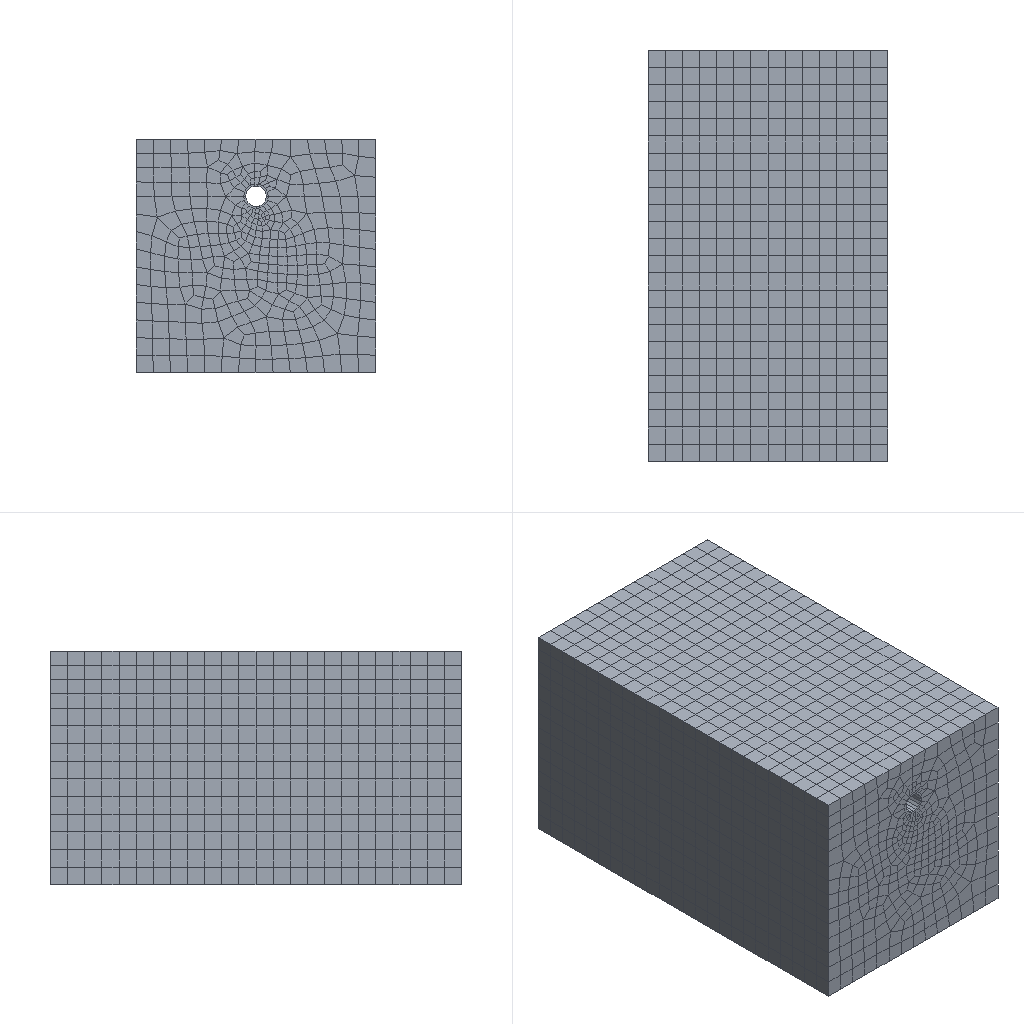Simulation study | abaqus
Set-up summary:
category,name,step,type,value,unit,region
solver,abaqus
solver,version,,,Abaqus/Standard 3DEXPERIENCE R2017x
units,not stated in the deck,,not stated
analysis,deck,,soils,soils
load_step,Step-2,Step-2,soils,nlgeom=False
contact,interactions,,,general=0 pairs=0 ties=0
load_step,requested,,,1
mesh,nodes,,,10350
mesh,elements,,,9048
element_type,C3D8R,,solid,456
element_type,C3D8RP,,solid,8592
load,load commands in deck,,count,2
bc,support commands in deck,,count,4
material,CHENQI,,in results
material,DAOCHUANG,,in results
material,FENTU,,in results
material,SHATU,,in results
check,setup vs results,,match,"per instance, exact: element labels, types and connectivity; labels of the nodes the elements use; coordinates of those nodes at SINGLE_PRECISION in 1 of 1 instance(s)"
Abaqus input file, long lists of numbers shortened:
*Heading
** Job name: Job-5 Model name: 100kmh
** Generated by: Abaqus/CAE 2017
*Preprint, echo=NO, model=NO, history=NO, contact=NO
**
** PARTS
**
*Part, name=work-2
*Node
      1,    2.65,         105.,   51.6
      2,    2.65,         -15.,   51.6
** (10348 more lines like these left out)
*Element, type=C3D8R
  1,   1,  23, 437,  86,   5,  87, 644, 145
  2,  23,  24, 438, 437,  87,  88, 645, 644
** (454 more lines like these left out)
*Element, type=C3D8RP
 457, 1251, 1244, 1236, 1247, 3230, 3223, 3215, 3226
 458, 1227, 1220,   83, 1219, 3206, 3199,  506, 3198
** (8590 more lines like these left out)
*Nset, nset=Set-10
     1,     2,     3,     4,     5,     6,     8,    10,    11,    14,    15,    18,    19,    20,    21,    22
    23,    24,    25,    26,    27,    28,    29,    30,    31,    32,    33,    34,    35,    36,    37,    38
** (172 more lines like these left out)
*Elset, elset=Set-10
  241,  242,  243,  244,  245,  246,  247,  248,  249,  250,  251,  252,  253,  254,  255,  256
  257,  258,  259,  260,  261,  262,  263,  264,  265,  266,  267,  268,  269,  270,  271,  272
** (130 more lines like these left out)
*Nset, nset=Set-11
     1,     2,     3,     4,     5,     6,     8,    10,    11,    14,    15,    18,    19,    20,    21,    22
    23,    24,    25,    26,    27,    28,    29,    30,    31,    32,    33,    34,    35,    36,    37,    38
** (172 more lines like these left out)
*Elset, elset=Set-11
  241,  242,  243,  244,  245,  246,  247,  248,  249,  250,  251,  252,  253,  254,  255,  256
  257,  258,  259,  260,  261,  262,  263,  264,  265,  266,  267,  268,  269,  270,  271,  272
** (130 more lines like these left out)
*Nset, nset=Set-12
    1,    2,    3,    4,    5,    6,    7,    8,    9,   10,   11,   12,   13,   14,   15,   16
   17,   18,   23,   24,   25,   26,   27,   28,   29,   30,   31,   32,   33,   34,   35,   36
** (497 more lines like these left out)
*Elset, elset=Set-12
    1,    2,    3,    4,    5,    6,    7,    8,    9,   10,   11,   12,   13,   14,   15,   16
   17,   18,   19,   20,   21,   22,   23,   24,   25,   26,   27,   28,   29,   30,   31,   32
** (432 more lines like these left out)
*Nset, nset=Set-13
     1,     2,     3,     4,    11,    14,    15,    18,    19,    20,    21,    22,    23,    24,    25,    26
    27,    28,    29,    30,    31,    32,    33,    34,    35,    36,    37,    38,    39,    40,    41,    42
** (156 more lines like these left out)
*Elset, elset=Set-13, generate
 7153,  9048,     1
*Nset, nset=Set-14
    1,    2,    3,    4,   11,   12,   13,   14,   15,   16,   17,   18,   23,   24,   25,   26
   27,   28,   29,   30,   31,   32,   33,   34,   35,   36,   37,   38,   39,   40,   41,   42
** (480 more lines like these left out)
*Elset, elset=Set-14, generate
  457,  7152,     1
*Nset, nset=Set-15
    1,    2,    3,    4,    5,    6,    7,    8,    9,   10,   23,   24,   25,   26,   27,   28
   29,   30,   31,   32,   33,   34,   35,   36,   37,   38,   39,   40,   41,   42,   43,   44
** (58 more lines like these left out)
*Elset, elset=Set-15, generate
   1,  456,    1
** Section: cq
*Solid Section, elset=Set-15, material=CHENQI
,
** Section: fs
*Solid Section, elset=Set-14, material=SHATU
,
** Section: f
*Solid Section, elset=Set-13, material=FENTU
,
*End Part
**
**
** ASSEMBLY
**
*Assembly, name=Assembly
**
*Instance, name=work-2-1, part=work-2
       -6.25,          15.,        -68.3
*End Instance
**
*Nset, nset=Set-1, instance=work-2-1, generate
     1,  10350,      1
*Elset, elset=Set-1, instance=work-2-1, generate
    1,  9048,     1
*Nset, nset=Set-2, instance=work-2-1, generate
     1,  10350,      1
*Elset, elset=Set-2, instance=work-2-1, generate
    1,  9048,     1
*Nset, nset=Set-3, instance=work-2-1
   19,   20,   21,   22,  358,  359,  360,  361,  362,  363,  364,  365,  366,  367,  368,  369
  370,  373,  374,  375,  376,  377,  378,  379,  380,  381,  382,  383,  384,  385,  386,  387
** (22 more lines like these left out)
*Elset, elset=Set-3, instance=work-2-1
 7159, 7163, 7168, 7177, 7179, 7181, 7199, 7202, 7205, 7206, 7210, 7215, 7216, 7222, 7238, 7242
 7247, 7256, 7258, 7260, 7278, 7281, 7284, 7285, 7289, 7294, 7295, 7301, 7317, 7321, 7326, 7335
** (19 more lines like these left out)
*Nset, nset=Set-4, instance=work-2-1
     1,     2,     3,     4,    11,    12,    13,    14,    15,    16,    17,    18,    19,    20,    21,    22
    23,    24,    25,    26,    27,    28,    29,    30,    31,    32,    33,    34,    35,    36,    37,    38
** (616 more lines like these left out)
*Elset, elset=Set-4, instance=work-2-1, generate
  457,  9048,     1
*Nset, nset=Set-5, instance=work-2-1, generate
     1,  10350,      1
*Elset, elset=Set-5, instance=work-2-1, generate
    1,  9048,     1
*Nset, nset=Set-6, instance=work-2-1
     1,     2,     3,     4,    11,    12,    13,    14,    15,    16,    17,    18,    19,    20,    21,    22
    23,    24,    25,    26,    27,    28,    29,    30,    31,    32,    33,    34,    35,    36,    37,    38
** (616 more lines like these left out)
*Elset, elset=Set-6, instance=work-2-1, generate
    1,  9048,     1
*Nset, nset=Set-7, instance=work-2-1
   12,   13,   16,   17,  195,  196,  197,  198,  199,  200,  201,  202,  203,  204,  205,  206
  207,  245,  246,  247,  248,  249,  250,  251,  252,  253,  254,  255,  256,  257,  258,  259
** (22 more lines like these left out)
*Elset, elset=Set-7, instance=work-2-1
  472,  474,  488,  489,  668,  673,  677,  687,  691,  695,  697,  698,  699,  701,  751,  753
  767,  768,  947,  952,  956,  966,  970,  974,  976,  977,  978,  980, 1030, 1032, 1046, 1047
** (19 more lines like these left out)
*Nset, nset=Set-8, instance=work-2-1
    1,    2,    3,    4,    5,    6,    7,    8,    9,   10,   11,   12,   13,   14,   15,   16
   17,   18,   19,   20,   21,   22,   46,   47,   48,   49,   50,   51,   52,   53,   54,   78
** (50 more lines like these left out)
*Elset, elset=Set-8, instance=work-2-1
    1,   24,   25,   48,   49,   72,   73,   96,   97,  120,  121,  144,  145,  168,  169,  192
  193,  216,  217,  240,  241,  264,  265,  288,  289,  312,  313,  336,  337,  360,  361,  384
** (46 more lines like these left out)
*Nset, nset=Set-9, instance=work-2-1
   11,   12,   13,   14,   15,   16,   17,   18,   19,   20,   21,   22,  186,  187,  188,  189
  190,  191,  192,  193,  194,  208,  209,  210,  211,  212,  213,  214,  215,  216,  222,  223
** (44 more lines like these left out)
*Elset, elset=Set-9, instance=work-2-1
  471,  472,  473,  479,  487,  489,  494,  629,  636,  665,  679,  685,  688,  690,  692,  693
  696,  706,  707,  709,  750,  751,  752,  758,  766,  768,  773,  908,  915,  944,  958,  964
** (39 more lines like these left out)
*Elset, elset=_Surf-3_S5, internal, instance=work-2-1
 7159, 7163, 7168, 7215, 7216, 7238, 7242, 7247, 7294, 7295, 7317, 7321, 7326, 7373, 7374, 7396
 7400, 7405, 7452, 7453, 7475, 7479, 7484, 7531, 7532, 7554, 7558, 7563, 7610, 7611, 7633, 7637
** (6 more lines like these left out)
*Elset, elset=_Surf-3_S3, internal, instance=work-2-1
 7177, 7179, 7181, 7199, 7202, 7205, 7206, 7210, 7222, 7256, 7258, 7260, 7278, 7281, 7284, 7285
 7289, 7301, 7335, 7337, 7339, 7357, 7360, 7363, 7364, 7368, 7380, 7414, 7416, 7418, 7436, 7439
** (12 more lines like these left out)
*Surface, type=ELEMENT, name=Surf-3
_Surf-3_S5, S5
_Surf-3_S3, S3
*Elset, elset=_m_Surf-1_S2, internal, instance=work-2-1, generate
   1,  240,    1
*Elset, elset=_m_Surf-1_S5, internal, instance=work-2-1, generate
 241,  456,    1
*Surface, type=ELEMENT, name=m_Surf-1
_m_Surf-1_S2, S2
_m_Surf-1_S5, S5
*Nset, nset=Set-3_PP_, internal, instance=work-2-1
   19,   20,   21,   22,  358,  359,  360,  361,  362,  363,  364,  365,  366,  367,  368,  369
  370,  373,  374,  375,  376,  377,  378,  379,  380,  381,  382,  383,  384,  385,  386,  387
** (22 more lines like these left out)
*End Assembly
*Amplitude, name=Amp-1
             0.,              0.,             50.,              1.
**
** MATERIALS
**
*Material, name=CHENQI
*Density
2500.,
*Elastic
 3.45e+10, 0.2
*Material, name=DAOCHUANG
*Density
 2.5,
*Elastic
30000., 0.2
*Material, name=FENTU
*Density
1960.,
*Elastic
 8.1e+09, 0.3
*Permeability, specific=9800.
 1.8e-05, 0.55
*Permeability, Type=SATURATION
 0.2739, 0.08001
 0.2915, 0.08002
 0.3109, 0.08002
 0.3321, 0.08003
 0.3553, 0.08003
 0.3808, 0.08004
 0.4088, 0.08005
 0.4396, 0.08006
 0.4733, 0.08009
 0.5103, 0.08012
 0.5506, 0.08016
 0.5944, 0.08024
 0.6417,  0.08035
 0.692, 0.08057
 0.7449,  0.08097
  0.7992, 0.08184
 0.8533, 0.084
 0.9046, 0.09087
 0.9498,  0.1233
 0.984,  0.4099
       1.,        1.
*Sorption
-400., 0.08001
-380., 0.08002
-360., 0.08002
-340., 0.08003
-320., 0.08003
-300., 0.08004
-280., 0.08005
-260., 0.08006
-240., 0.08009
-220., 0.08012
-200., 0.08016
-180., 0.08024
-160.,  0.08035
-140., 0.08057
-120.,  0.08097
-100., 0.08184
 -80., 0.084
 -60., 0.09087
 -40.,  0.1233
 -20.,  0.4099
   0.,        1.
*Material, name=SHATU
*Density
2020.,
*Elastic
 1.263e+10, 0.3
*Permeability, specific=9800.
 1.8e-05, 0.55
*Permeability, Type=SATURATION
 0.2739, 0.08001
 0.2915, 0.08002
 0.3109, 0.08002
 0.3321, 0.08003
 0.3553, 0.08003
 0.3808, 0.08004
 0.4088, 0.08005
 0.4396, 0.08006
 0.4733, 0.08009
 0.5103, 0.08012
 0.5506, 0.08016
 0.5944, 0.08024
 0.6417,  0.08035
 0.692, 0.08057
 0.7449,  0.08097
  0.7992, 0.08184
 0.8533, 0.084
 0.9046, 0.09087
 0.9498,  0.1233
 0.984,  0.4099
       1.,        1.
*Sorption
-400., 0.08001
-380., 0.08002
-360., 0.08002
-340., 0.08003
-320., 0.08003
-300., 0.08004
-280., 0.08005
-260., 0.08006
-240., 0.08009
-220., 0.08012
-200., 0.08016
-180., 0.08024
-160.,  0.08035
-140., 0.08057
-120.,  0.08097
-100., 0.08184
 -80., 0.084
 -60., 0.09087
 -40.,  0.1233
 -20.,  0.4099
   0.,        1.
**
** PREDEFINED FIELDS
**
** Name: Predefined Field-2   Type: Void ratio
*Initial Conditions, TYPE=RATIO
Set-6, 0.3
** ----------------------------------------------------------------
**
** STEP: Step-2
**
*Step, name=Step-2, nlgeom=NO, inc=10000, unsymm=YES
*Soils, consolidation, end=PERIOD, utol=1e+17, creep=none
0.5, 50., 5e-05, 1.,
**
** BOUNDARY CONDITIONS
**
** Name: BC-1 Type: 孔隙压力
*Boundary
Set-3_PP_, 8, 8, 50.
** Name: BC-2 Type: 位移/转角
*Boundary
Set-7, 3, 3
** Name: BC-3 Type: 位移/转角
*Boundary
Set-8, 2, 2
** Name: BC-4 Type: 位移/转角
*Boundary
Set-9, 1, 1
**
** LOADS
**
** Name: Load-1   Type: Pressure
*Dsload
Surf-3, PNU, 1000.
**
** OUTPUT REQUESTS
**
*Restart, write, frequency=0
**
** FIELD OUTPUT: F-Output-1
**
*Output, field
*Node Output
CF, NT, POR, RF, RM, RT, TF, U
V
*Element Output, directions=YES
ALPHAN, DAMAGEC, DAMAGET, DMICRT, E, FLUVR, FLVEL, LE, MISES, MISESMAX, MISESONLY, NE, PE, PEEQ, PEEQMAX, PEEQT
PEMAG, PRESSONLY, PS, S, SAT, SDEG, SF, SSAVG, TEMP, VEEQ, VOIDR
*Contact Output
BDSTAT, CDISP, CSTRESS
*Output, history, frequency=0
*End Step
Results summary:
result,step,,completed,increments=52 time=50.0/50.0
result,analysis,,,"soils, consolidation"
result,last_loadstep,,,1
result,analysis steps,,count,1
result,primary field,,,"U, POR"
result,reaction total,,FX,8.4e-05,model units
result,reaction total,,FY,-0.000104,model units
result,reaction total,,FZ,1e-06,model units